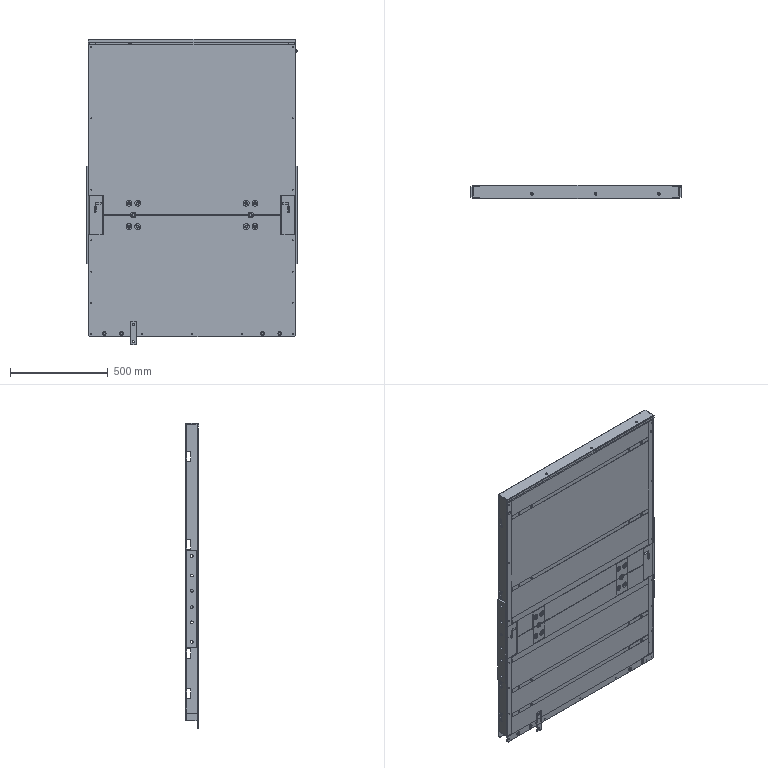Part | SolidWorks | 58 solids | 1694 faces | box 1080 x 70 x 1565 mm | volume 11988496 mm3 | plane 1006 | cylinder 586 | cone 102 | commonest cylinder face diameters 10 x90 14.5 x88 11 x84 0.4 x36 5 x34 20 x32